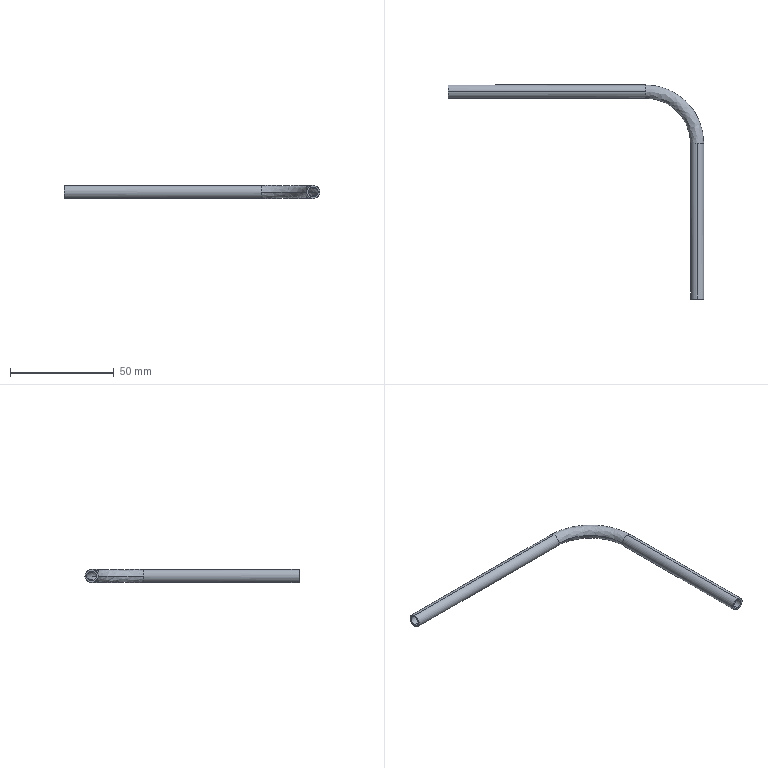Part | STEP file | copper tube 26_default_machined_ | 1 solid | 14 faces | box 123.175 x 103.175 x 6.35 mm | volume 2919 mm3 | cylinder 8 | spline 4 | plane 2 | commonest cylinder face diameters 4.75 x4 6.35 x4